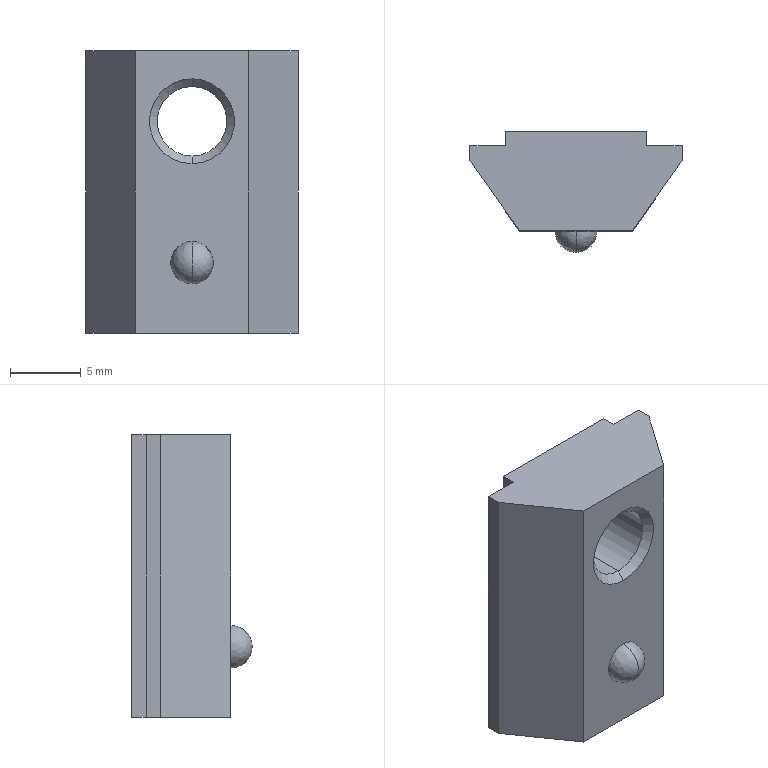Part | SolidWorks | features BaseBody 1 | 1 solid | 20 faces | box 15 x 8.5 x 20 mm | volume 1520 mm3 | plane 12 | cone 4 | spline 2 | cylinder 2 | commonest cylinder face diameters 4.917 x2
STEP:
#1=CARTESIAN_POINT('',(0.,0.,-13.5));
#2=VERTEX_POINT('',#1);
#3=CARTESIAN_POINT('',(0.,0.,-16.5));
#4=VERTEX_POINT('',#3);
#5=CARTESIAN_POINT('',(0.,0.,-15.));
#6=DIRECTION('',(0.,1.,0.));
#7=DIRECTION('',(0.,0.,1.));
#8=AXIS2_PLACEMENT_3D('',#5,#6,#7);
#9=CIRCLE('',#8,1.5);
#10=EDGE_CURVE('',#2,#4,#9,.T.);
#11=ORIENTED_EDGE('',*,*,#10,.F.);
#12=CARTESIAN_POINT('',(0.,-1.5,-15.));
#13=VERTEX_POINT('',#12);
#14=CARTESIAN_POINT('',(0.,0.,-15.));
#15=DIRECTION('',(1.,0.,0.));
#16=DIRECTION('',(0.,1.,0.));
#17=AXIS2_PLACEMENT_3D('',#14,#15,#16);
#18=CIRCLE('',#17,1.5);
#19=EDGE_CURVE('',#2,#13,#18,.T.);
#20=ORIENTED_EDGE('',*,*,#19,.T.);
#21=CARTESIAN_POINT('',(0.,0.,-15.));
#22=DIRECTION('',(-1.,0.,0.));
#23=DIRECTION('',(0.,1.,0.));
#24=AXIS2_PLACEMENT_3D('',#21,#22,#23);
#25=CIRCLE('',#24,1.5);
#26=EDGE_CURVE('',#4,#13,#25,.T.);
#27=ORIENTED_EDGE('',*,*,#26,.F.);
#28=EDGE_LOOP('',(#11,#20,#27));
#29=FACE_OUTER_BOUND('',#28,.T.);
#30=CARTESIAN_POINT('',(0.,0.,-13.5));
#31=CARTESIAN_POINT('',(3.,0.,-13.5));
#32=CARTESIAN_POINT('',(3.,0.,-16.5));
#33=CARTESIAN_POINT('',(0.,0.,-16.5));
#34=CARTESIAN_POINT('',(0.,-0.8787,-13.5));
#35=CARTESIAN_POINT('',(3.,-0.8787,-13.5));
#36=CARTESIAN_POINT('',(3.,-0.8787,-16.5));
#37=CARTESIAN_POINT('',(0.,-0.8787,-16.5));
#38=CARTESIAN_POINT('',(0.,-1.5,-14.121));
#39=CARTESIAN_POINT('',(1.757,-1.5,-14.121));
#40=CARTESIAN_POINT('',(1.757,-1.5,-15.879));
#41=CARTESIAN_POINT('',(0.,-1.5,-15.879));
#42=CARTESIAN_POINT('',(0.,-1.5,-15.));
#43=CARTESIAN_POINT('',(0.,-1.5,-15.));
#44=CARTESIAN_POINT('',(0.,-1.5,-15.));
#45=CARTESIAN_POINT('',(0.,-1.5,-15.));
#46=(BOUNDED_SURFACE()B_SPLINE_SURFACE(3,3,((#30,#31,#32,#33),(#34,#35,#36,#37),(#38,#39,#40,#41),(#42,#43,#44,#45)),.UNSPECIFIED.,.F.,.F.,.F.)B_SPLINE_SURFACE_WITH_KNOTS((4,4),(4,4),(0.,1.),(0.,1.),.UNSPECIFIED.)GEOMETRIC_REPRESENTATION_ITEM()RATIONAL_B_SPLINE_SURFACE(((1.,0.3333,0.3333,1.),(0.8047,0.2682,0.2682,0.8047),(0.8047,0.2682,0.2682,0.8047),(1.,0.3333,0.3333,1.)))REPRESENTATION_ITEM('')SURFACE());
#47=ADVANCED_FACE('',(#29),#46,.T.);
#48=CARTESIAN_POINT('',(0.,6.459,-7.458));
#49=VERTEX_POINT('',#48);
#50=CARTESIAN_POINT('',(0.,6.459,-2.542));
#51=VERTEX_POINT('',#50);
#52=CARTESIAN_POINT('',(0.,6.459,-5.));
#53=DIRECTION('',(0.,1.,0.));
#54=DIRECTION('',(0.,0.,1.));
#55=AXIS2_PLACEMENT_3D('',#52,#53,#54);
#56=CIRCLE('',#55,2.458);
#57=EDGE_CURVE('',#49,#51,#56,.T.);
#58=ORIENTED_EDGE('',*,*,#57,.F.);
#59=CARTESIAN_POINT('',(0.,7.,-8.));
#60=VERTEX_POINT('',#59);
#61=CARTESIAN_POINT('',(0.,7.,-8.));
#62=DIRECTION('',(0.,0.7071,-0.7071));
#63=VECTOR('',#62,1000.);
#64=LINE('',#61,#63);
#65=EDGE_CURVE('',#49,#60,#64,.T.);
#66=ORIENTED_EDGE('',*,*,#65,.T.);
#67=CARTESIAN_POINT('',(0.,7.,-2.));
#68=VERTEX_POINT('',#67);
#69=CARTESIAN_POINT('',(0.,7.,-5.));
#70=DIRECTION('',(0.,-1.,0.));
#71=DIRECTION('',(0.,0.,1.));
#72=AXIS2_PLACEMENT_3D('',#69,#70,#71);
#73=CIRCLE('',#72,3.);
#74=EDGE_CURVE('',#68,#60,#73,.T.);
#75=ORIENTED_EDGE('',*,*,#74,.F.);
#76=CARTESIAN_POINT('',(0.,7.,-2.));
#77=DIRECTION('',(0.,0.7071,0.7071));
#78=VECTOR('',#77,1000.);
#79=LINE('',#76,#78);
#80=EDGE_CURVE('',#51,#68,#79,.T.);
#81=ORIENTED_EDGE('',*,*,#80,.F.);
#82=EDGE_LOOP('',(#58,#66,#75,#81));
#83=FACE_OUTER_BOUND('',#82,.T.);
#84=CARTESIAN_POINT('',(0.,7.,-5.));
#85=DIRECTION('',(0.,1.,0.));
#86=DIRECTION('',(0.,0.,1.));
#87=AXIS2_PLACEMENT_3D('',#84,#85,#86);
#88=CONICAL_SURFACE('',#87,3.,0.7854);
#89=ADVANCED_FACE('',(#83),#88,.F.);
#90=CARTESIAN_POINT('',(0.,0.5415,-7.458));
#91=VERTEX_POINT('',#90);
#92=CARTESIAN_POINT('',(0.,0.5415,-2.542));
#93=VERTEX_POINT('',#92);
#94=CARTESIAN_POINT('',(0.,0.5415,-5.));
#95=DIRECTION('',(0.,1.,0.));
#96=DIRECTION('',(0.,0.,1.));
#97=AXIS2_PLACEMENT_3D('',#94,#95,#96);
#98=CIRCLE('',#97,2.458);
#99=EDGE_CURVE('',#91,#93,#98,.T.);
#100=ORIENTED_EDGE('',*,*,#99,.F.);
#101=CARTESIAN_POINT('',(0.,0.,-7.458));
#102=DIRECTION('',(0.,1.,0.));
#103=VECTOR('',#102,1000.);
#104=LINE('',#101,#103);
#105=EDGE_CURVE('',#91,#49,#104,.T.);
#106=ORIENTED_EDGE('',*,*,#105,.T.);
#107=ORIENTED_EDGE('',*,*,#57,.T.);
#108=CARTESIAN_POINT('',(0.,0.,-2.542));
#109=DIRECTION('',(0.,1.,0.));
#110=VECTOR('',#109,1000.);
#111=LINE('',#108,#110);
#112=EDGE_CURVE('',#93,#51,#111,.T.);
#113=ORIENTED_EDGE('',*,*,#112,.F.);
#114=EDGE_LOOP('',(#100,#106,#107,#113));
#115=FACE_OUTER_BOUND('',#114,.T.);
#116=CARTESIAN_POINT('',(0.,0.,-5.));
#117=DIRECTION('',(0.,1.,0.));
#118=DIRECTION('',(0.,0.,1.));
#119=AXIS2_PLACEMENT_3D('',#116,#117,#118);
#120=CYLINDRICAL_SURFACE('',#119,2.458);
#121=ADVANCED_FACE('',(#115),#120,.F.);
#122=ORIENTED_EDGE('',*,*,#99,.T.);
#123=CARTESIAN_POINT('',(0.,0.,-2.));
#124=VERTEX_POINT('',#123);
#125=CARTESIAN_POINT('',(0.,0.,-2.));
#126=DIRECTION('',(0.,-0.7071,0.7071));
#127=VECTOR('',#126,1000.);
#128=LINE('',#125,#127);
#129=EDGE_CURVE('',#93,#124,#128,.T.);
#130=ORIENTED_EDGE('',*,*,#129,.T.);
#131=CARTESIAN_POINT('',(0.,0.,-8.));
#132=VERTEX_POINT('',#131);
#133=CARTESIAN_POINT('',(0.,0.,-5.));
#134=DIRECTION('',(0.,1.,0.));
#135=DIRECTION('',(0.,0.,-1.));
#136=AXIS2_PLACEMENT_3D('',#133,#134,#135);
#137=CIRCLE('',#136,3.);
#138=EDGE_CURVE('',#132,#124,#137,.T.);
#139=ORIENTED_EDGE('',*,*,#138,.F.);
#140=CARTESIAN_POINT('',(0.,0.,-8.));
#141=DIRECTION('',(0.,-0.7071,-0.7071));
#142=VECTOR('',#141,1000.);
#143=LINE('',#140,#142);
#144=EDGE_CURVE('',#91,#132,#143,.T.);
#145=ORIENTED_EDGE('',*,*,#144,.F.);
#146=EDGE_LOOP('',(#122,#130,#139,#145));
#147=FACE_OUTER_BOUND('',#146,.T.);
#148=CARTESIAN_POINT('',(0.,0.,-5.));
#149=DIRECTION('',(0.,-1.,0.));
#150=DIRECTION('',(0.,0.,-1.));
#151=AXIS2_PLACEMENT_3D('',#148,#149,#150);
#152=CONICAL_SURFACE('',#151,3.,0.7854);
#153=ADVANCED_FACE('',(#147),#152,.F.);
#154=ORIENTED_EDGE('',*,*,#74,.T.);
#155=CARTESIAN_POINT('',(0.,7.,-5.));
#156=DIRECTION('',(0.,-1.,0.));
#157=DIRECTION('',(0.,0.,1.));
#158=AXIS2_PLACEMENT_3D('',#155,#156,#157);
#159=CIRCLE('',#158,3.);
#160=EDGE_CURVE('',#60,#68,#159,.T.);
#161=ORIENTED_EDGE('',*,*,#160,.T.);
#162=EDGE_LOOP('',(#154,#161));
#163=FACE_BOUND('',#162,.T.);
#164=CARTESIAN_POINT('',(5.,7.,-20.));
#165=VERTEX_POINT('',#164);
#166=CARTESIAN_POINT('',(-5.,7.,-20.));
#167=VERTEX_POINT('',#166);
#168=CARTESIAN_POINT('',(5.,7.,-20.));
#169=DIRECTION('',(-1.,0.,0.));
#170=VECTOR('',#169,1000.);
#171=LINE('',#168,#170);
#172=EDGE_CURVE('',#165,#167,#171,.T.);
#173=ORIENTED_EDGE('',*,*,#172,.T.);
#174=CARTESIAN_POINT('',(-5.,7.,0.));
#175=VERTEX_POINT('',#174);
#176=CARTESIAN_POINT('',(-5.,7.,-20.));
#177=DIRECTION('',(0.,0.,1.));
#178=VECTOR('',#177,1000.);
#179=LINE('',#176,#178);
#180=EDGE_CURVE('',#167,#175,#179,.T.);
#181=ORIENTED_EDGE('',*,*,#180,.T.);
#182=CARTESIAN_POINT('',(5.,7.,0.));
#183=VERTEX_POINT('',#182);
#184=CARTESIAN_POINT('',(5.,7.,0.));
#185=DIRECTION('',(1.,0.,0.));
#186=VECTOR('',#185,1000.);
#187=LINE('',#184,#186);
#188=EDGE_CURVE('',#175,#183,#187,.T.);
#189=ORIENTED_EDGE('',*,*,#188,.T.);
#190=CARTESIAN_POINT('',(5.,7.,-20.));
#191=DIRECTION('',(0.,0.,-1.));
#192=VECTOR('',#191,1000.);
#193=LINE('',#190,#192);
#194=EDGE_CURVE('',#183,#165,#193,.T.);
#195=ORIENTED_EDGE('',*,*,#194,.T.);
#196=EDGE_LOOP('',(#173,#181,#189,#195));
#197=FACE_OUTER_BOUND('',#196,.T.);
#198=CARTESIAN_POINT('',(5.,7.,-20.));
#199=DIRECTION('',(0.,1.,0.));
#200=DIRECTION('',(0.,0.,1.));
#201=AXIS2_PLACEMENT_3D('',#198,#199,#200);
#202=PLANE('',#201);
#203=ADVANCED_FACE('',(#163,#197),#202,.T.);
#204=ORIENTED_EDGE('',*,*,#65,.F.);
#205=CARTESIAN_POINT('',(0.,6.459,-5.));
#206=DIRECTION('',(0.,1.,0.));
#207=DIRECTION('',(0.,0.,1.));
#208=AXIS2_PLACEMENT_3D('',#205,#206,#207);
#209=CIRCLE('',#208,2.458);
#210=EDGE_CURVE('',#51,#49,#209,.T.);
#211=ORIENTED_EDGE('',*,*,#210,.F.);
#212=ORIENTED_EDGE('',*,*,#80,.T.);
#213=ORIENTED_EDGE('',*,*,#160,.F.);
#214=EDGE_LOOP('',(#204,#211,#212,#213));
#215=FACE_OUTER_BOUND('',#214,.T.);
#216=CARTESIAN_POINT('',(0.,7.,-5.));
#217=DIRECTION('',(0.,1.,0.));
#218=DIRECTION('',(0.,0.,1.));
#219=AXIS2_PLACEMENT_3D('',#216,#217,#218);
#220=CONICAL_SURFACE('',#219,3.,0.7854);
#221=ADVANCED_FACE('',(#215),#220,.F.);
#222=CARTESIAN_POINT('',(-5.,6.,-20.));
#223=VERTEX_POINT('',#222);
#224=CARTESIAN_POINT('',(-5.,7.,-20.));
#225=DIRECTION('',(0.,-1.,0.));
#226=VECTOR('',#225,1000.);
#227=LINE('',#224,#226);
#228=EDGE_CURVE('',#167,#223,#227,.T.);
#229=ORIENTED_EDGE('',*,*,#228,.T.);
#230=CARTESIAN_POINT('',(-5.,6.,0.));
#231=VERTEX_POINT('',#230);
#232=CARTESIAN_POINT('',(-5.,6.,-20.));
#233=DIRECTION('',(0.,0.,1.));
#234=VECTOR('',#233,1000.);
#235=LINE('',#232,#234);
#236=EDGE_CURVE('',#223,#231,#235,.T.);
#237=ORIENTED_EDGE('',*,*,#236,.T.);
#238=CARTESIAN_POINT('',(-5.,7.,0.));
#239=DIRECTION('',(0.,1.,0.));
#240=VECTOR('',#239,1000.);
#241=LINE('',#238,#240);
#242=EDGE_CURVE('',#231,#175,#241,.T.);
#243=ORIENTED_EDGE('',*,*,#242,.T.);
#244=ORIENTED_EDGE('',*,*,#180,.F.);
#245=EDGE_LOOP('',(#229,#237,#243,#244));
#246=FACE_OUTER_BOUND('',#245,.T.);
#247=CARTESIAN_POINT('',(-5.,7.,-20.));
#248=DIRECTION('',(-1.,0.,0.));
#249=DIRECTION('',(0.,0.,1.));
#250=AXIS2_PLACEMENT_3D('',#247,#248,#249);
#251=PLANE('',#250);
#252=ADVANCED_FACE('',(#246),#251,.T.);
#253=CARTESIAN_POINT('',(-7.5,6.,-20.));
#254=VERTEX_POINT('',#253);
#255=CARTESIAN_POINT('',(0.,6.,-20.));
#256=DIRECTION('',(-1.,0.,0.));
#257=VECTOR('',#256,1000.);
#258=LINE('',#255,#257);
#259=EDGE_CURVE('',#223,#254,#258,.T.);
#260=ORIENTED_EDGE('',*,*,#259,.F.);
#261=ORIENTED_EDGE('',*,*,#228,.F.);
#262=ORIENTED_EDGE('',*,*,#172,.F.);
#263=CARTESIAN_POINT('',(5.,6.,-20.));
#264=VERTEX_POINT('',#263);
#265=CARTESIAN_POINT('',(5.,0.,-20.));
#266=DIRECTION('',(0.,1.,0.));
#267=VECTOR('',#266,1000.);
#268=LINE('',#265,#267);
#269=EDGE_CURVE('',#264,#165,#268,.T.);
#270=ORIENTED_EDGE('',*,*,#269,.F.);
#271=CARTESIAN_POINT('',(7.5,6.,-20.));
#272=VERTEX_POINT('',#271);
#273=CARTESIAN_POINT('',(0.,6.,-20.));
#274=DIRECTION('',(-1.,0.,0.));
#275=VECTOR('',#274,1000.);
#276=LINE('',#273,#275);
#277=EDGE_CURVE('',#272,#264,#276,.T.);
#278=ORIENTED_EDGE('',*,*,#277,.F.);
#279=CARTESIAN_POINT('',(7.5,4.979,-20.));
#280=VERTEX_POINT('',#279);
#281=CARTESIAN_POINT('',(7.5,4.979,-20.));
#282=DIRECTION('',(0.,1.,0.));
#283=VECTOR('',#282,1000.);
#284=LINE('',#281,#283);
#285=EDGE_CURVE('',#280,#272,#284,.T.);
#286=ORIENTED_EDGE('',*,*,#285,.F.);
#287=CARTESIAN_POINT('',(4.,0.,-20.));
#288=VERTEX_POINT('',#287);
#289=CARTESIAN_POINT('',(4.,0.,-20.));
#290=DIRECTION('',(0.5751,0.8181,0.));
#291=VECTOR('',#290,1000.);
#292=LINE('',#289,#291);
#293=EDGE_CURVE('',#288,#280,#292,.T.);
#294=ORIENTED_EDGE('',*,*,#293,.F.);
#295=CARTESIAN_POINT('',(-4.,0.,-20.));
#296=VERTEX_POINT('',#295);
#297=CARTESIAN_POINT('',(0.,0.,-20.));
#298=DIRECTION('',(1.,0.,0.));
#299=VECTOR('',#298,1000.);
#300=LINE('',#297,#299);
#301=EDGE_CURVE('',#296,#288,#300,.T.);
#302=ORIENTED_EDGE('',*,*,#301,.F.);
#303=CARTESIAN_POINT('',(-7.5,5.,-20.));
#304=VERTEX_POINT('',#303);
#305=CARTESIAN_POINT('',(-7.5,5.,-20.));
#306=DIRECTION('',(0.5735,-0.8192,0.));
#307=VECTOR('',#306,1000.);
#308=LINE('',#305,#307);
#309=EDGE_CURVE('',#304,#296,#308,.T.);
#310=ORIENTED_EDGE('',*,*,#309,.F.);
#311=CARTESIAN_POINT('',(-7.5,6.,-20.));
#312=DIRECTION('',(0.,-1.,0.));
#313=VECTOR('',#312,1000.);
#314=LINE('',#311,#313);
#315=EDGE_CURVE('',#254,#304,#314,.T.);
#316=ORIENTED_EDGE('',*,*,#315,.F.);
#317=EDGE_LOOP('',(#260,#261,#262,#270,#278,#286,#294,#302,#310,#316));
#318=FACE_OUTER_BOUND('',#317,.T.);
#319=CARTESIAN_POINT('',(0.,0.,-20.));
#320=DIRECTION('',(0.,0.,1.));
#321=DIRECTION('',(1.,0.,0.));
#322=AXIS2_PLACEMENT_3D('',#319,#320,#321);
#323=PLANE('',#322);
#324=ADVANCED_FACE('',(#318),#323,.F.);
#325=ORIENTED_EDGE('',*,*,#269,.T.);
#326=ORIENTED_EDGE('',*,*,#194,.F.);
#327=CARTESIAN_POINT('',(5.,6.,0.));
#328=VERTEX_POINT('',#327);
#329=CARTESIAN_POINT('',(5.,6.,0.));
#330=DIRECTION('',(0.,-1.,0.));
#331=VECTOR('',#330,1000.);
#332=LINE('',#329,#331);
#333=EDGE_CURVE('',#183,#328,#332,.T.);
#334=ORIENTED_EDGE('',*,*,#333,.T.);
#335=CARTESIAN_POINT('',(5.,6.,-20.));
#336=DIRECTION('',(0.,0.,-1.));
#337=VECTOR('',#336,1000.);
#338=LINE('',#335,#337);
#339=EDGE_CURVE('',#328,#264,#338,.T.);
#340=ORIENTED_EDGE('',*,*,#339,.T.);
#341=EDGE_LOOP('',(#325,#326,#334,#340));
#342=FACE_OUTER_BOUND('',#341,.T.);
#343=CARTESIAN_POINT('',(5.,6.,-20.));
#344=DIRECTION('',(1.,0.,0.));
#345=DIRECTION('',(0.,0.,-1.));
#346=AXIS2_PLACEMENT_3D('',#343,#344,#345);
#347=PLANE('',#346);
#348=ADVANCED_FACE('',(#342),#347,.T.);
#349=ORIENTED_EDGE('',*,*,#242,.F.);
#350=CARTESIAN_POINT('',(-7.5,6.,0.));
#351=VERTEX_POINT('',#350);
#352=CARTESIAN_POINT('',(0.,6.,0.));
#353=DIRECTION('',(-1.,0.,0.));
#354=VECTOR('',#353,1000.);
#355=LINE('',#352,#354);
#356=EDGE_CURVE('',#231,#351,#355,.T.);
#357=ORIENTED_EDGE('',*,*,#356,.T.);
#358=CARTESIAN_POINT('',(-7.5,5.,0.));
#359=VERTEX_POINT('',#358);
#360=CARTESIAN_POINT('',(-7.5,6.,0.));
#361=DIRECTION('',(0.,1.,0.));
#362=VECTOR('',#361,1000.);
#363=LINE('',#360,#362);
#364=EDGE_CURVE('',#359,#351,#363,.T.);
#365=ORIENTED_EDGE('',*,*,#364,.F.);
#366=CARTESIAN_POINT('',(-4.,0.,0.));
#367=VERTEX_POINT('',#366);
#368=CARTESIAN_POINT('',(-7.5,5.,0.));
#369=DIRECTION('',(0.5735,-0.8192,0.));
#370=VECTOR('',#369,1000.);
#371=LINE('',#368,#370);
#372=EDGE_CURVE('',#359,#367,#371,.T.);
#373=ORIENTED_EDGE('',*,*,#372,.T.);
#374=CARTESIAN_POINT('',(4.,0.,0.));
#375=VERTEX_POINT('',#374);
#376=CARTESIAN_POINT('',(0.,0.,0.));
#377=DIRECTION('',(1.,0.,0.));
#378=VECTOR('',#377,1000.);
#379=LINE('',#376,#378);
#380=EDGE_CURVE('',#367,#375,#379,.T.);
#381=ORIENTED_EDGE('',*,*,#380,.T.);
#382=CARTESIAN_POINT('',(7.5,4.979,0.));
#383=VERTEX_POINT('',#382);
#384=CARTESIAN_POINT('',(4.,0.,0.));
#385=DIRECTION('',(0.5751,0.8181,0.));
#386=VECTOR('',#385,1000.);
#387=LINE('',#384,#386);
#388=EDGE_CURVE('',#375,#383,#387,.T.);
#389=ORIENTED_EDGE('',*,*,#388,.T.);
#390=CARTESIAN_POINT('',(7.5,6.,0.));
#391=VERTEX_POINT('',#390);
#392=CARTESIAN_POINT('',(7.5,4.979,0.));
#393=DIRECTION('',(0.,-1.,0.));
#394=VECTOR('',#393,1000.);
#395=LINE('',#392,#394);
#396=EDGE_CURVE('',#391,#383,#395,.T.);
#397=ORIENTED_EDGE('',*,*,#396,.F.);
#398=CARTESIAN_POINT('',(0.,6.,0.));
#399=DIRECTION('',(-1.,0.,0.));
#400=VECTOR('',#399,1000.);
#401=LINE('',#398,#400);
#402=EDGE_CURVE('',#391,#328,#401,.T.);
#403=ORIENTED_EDGE('',*,*,#402,.T.);
#404=ORIENTED_EDGE('',*,*,#333,.F.);
#405=ORIENTED_EDGE('',*,*,#188,.F.);
#406=EDGE_LOOP('',(#349,#357,#365,#373,#381,#389,#397,#403,#404,#405));
#407=FACE_OUTER_BOUND('',#406,.T.);
#408=CARTESIAN_POINT('',(0.,0.,0.));
#409=DIRECTION('',(0.,0.,1.));
#410=DIRECTION('',(1.,0.,0.));
#411=AXIS2_PLACEMENT_3D('',#408,#409,#410);
#412=PLANE('',#411);
#413=ADVANCED_FACE('',(#407),#412,.T.);
#414=ORIENTED_EDGE('',*,*,#105,.F.);
#415=CARTESIAN_POINT('',(0.,0.5415,-5.));
#416=DIRECTION('',(0.,1.,0.));
#417=DIRECTION('',(0.,0.,1.));
#418=AXIS2_PLACEMENT_3D('',#415,#416,#417);
#419=CIRCLE('',#418,2.458);
#420=EDGE_CURVE('',#93,#91,#419,.T.);
#421=ORIENTED_EDGE('',*,*,#420,.F.);
#422=ORIENTED_EDGE('',*,*,#112,.T.);
#423=ORIENTED_EDGE('',*,*,#210,.T.);
#424=EDGE_LOOP('',(#414,#421,#422,#423));
#425=FACE_OUTER_BOUND('',#424,.T.);
#426=CARTESIAN_POINT('',(0.,0.,-5.));
#427=DIRECTION('',(0.,1.,0.));
#428=DIRECTION('',(0.,0.,1.));
#429=AXIS2_PLACEMENT_3D('',#426,#427,#428);
#430=CYLINDRICAL_SURFACE('',#429,2.458);
#431=ADVANCED_FACE('',(#425),#430,.F.);
#432=ORIENTED_EDGE('',*,*,#259,.T.);
#433=CARTESIAN_POINT('',(-7.5,6.,-20.));
#434=DIRECTION('',(0.,0.,1.));
#435=VECTOR('',#434,1000.);
#436=LINE('',#433,#435);
#437=EDGE_CURVE('',#254,#351,#436,.T.);
#438=ORIENTED_EDGE('',*,*,#437,.T.);
#439=ORIENTED_EDGE('',*,*,#356,.F.);
#440=ORIENTED_EDGE('',*,*,#236,.F.);
#441=EDGE_LOOP('',(#432,#438,#439,#440));
#442=FACE_OUTER_BOUND('',#441,.T.);
#443=CARTESIAN_POINT('',(-5.,6.,-20.));
#444=DIRECTION('',(0.,1.,0.));
#445=DIRECTION('',(0.,0.,1.));
#446=AXIS2_PLACEMENT_3D('',#443,#444,#445);
#447=PLANE('',#446);
#448=ADVANCED_FACE('',(#442),#447,.T.);
#449=ORIENTED_EDGE('',*,*,#277,.T.);
#450=ORIENTED_EDGE('',*,*,#339,.F.);
#451=ORIENTED_EDGE('',*,*,#402,.F.);
#452=CARTESIAN_POINT('',(7.5,6.,-20.));
#453=DIRECTION('',(0.,0.,-1.));
#454=VECTOR('',#453,1000.);
#455=LINE('',#452,#454);
#456=EDGE_CURVE('',#391,#272,#455,.T.);
#457=ORIENTED_EDGE('',*,*,#456,.T.);
#458=EDGE_LOOP('',(#449,#450,#451,#457));
#459=FACE_OUTER_BOUND('',#458,.T.);
#460=CARTESIAN_POINT('',(7.5,6.,-20.));
#461=DIRECTION('',(0.,1.,0.));
#462=DIRECTION('',(0.,0.,1.));
#463=AXIS2_PLACEMENT_3D('',#460,#461,#462);
#464=PLANE('',#463);
#465=ADVANCED_FACE('',(#459),#464,.T.);
#466=ORIENTED_EDGE('',*,*,#293,.T.);
#467=CARTESIAN_POINT('',(7.5,4.979,-20.));
#468=DIRECTION('',(0.,0.,1.));
#469=VECTOR('',#468,1000.);
#470=LINE('',#467,#469);
#471=EDGE_CURVE('',#280,#383,#470,.T.);
#472=ORIENTED_EDGE('',*,*,#471,.T.);
#473=ORIENTED_EDGE('',*,*,#388,.F.);
#474=CARTESIAN_POINT('',(4.,0.,-20.));
#475=DIRECTION('',(0.,0.,-1.));
#476=VECTOR('',#475,1000.);
#477=LINE('',#474,#476);
#478=EDGE_CURVE('',#375,#288,#477,.T.);
#479=ORIENTED_EDGE('',*,*,#478,.T.);
#480=EDGE_LOOP('',(#466,#472,#473,#479));
#481=FACE_OUTER_BOUND('',#480,.T.);
#482=CARTESIAN_POINT('',(4.,0.,-20.));
#483=DIRECTION('',(0.8181,-0.5751,0.));
#484=DIRECTION('',(0.5751,0.8181,0.));
#485=AXIS2_PLACEMENT_3D('',#482,#483,#484);
#486=PLANE('',#485);
#487=ADVANCED_FACE('',(#481),#486,.T.);
#488=ORIENTED_EDGE('',*,*,#138,.T.);
#489=CARTESIAN_POINT('',(0.,0.,-5.));
#490=DIRECTION('',(0.,1.,0.));
#491=DIRECTION('',(0.,0.,-1.));
#492=AXIS2_PLACEMENT_3D('',#489,#490,#491);
#493=CIRCLE('',#492,3.);
#494=EDGE_CURVE('',#124,#132,#493,.T.);
#495=ORIENTED_EDGE('',*,*,#494,.T.);
#496=EDGE_LOOP('',(#488,#495));
#497=FACE_BOUND('',#496,.T.);
#498=ORIENTED_EDGE('',*,*,#301,.T.);
#499=ORIENTED_EDGE('',*,*,#478,.F.);
#500=ORIENTED_EDGE('',*,*,#380,.F.);
#501=CARTESIAN_POINT('',(-4.,0.,-20.));
#502=DIRECTION('',(0.,0.,-1.));
#503=VECTOR('',#502,1000.);
#504=LINE('',#501,#503);
#505=EDGE_CURVE('',#367,#296,#504,.T.);
#506=ORIENTED_EDGE('',*,*,#505,.T.);
#507=EDGE_LOOP('',(#498,#499,#500,#506));
#508=FACE_OUTER_BOUND('',#507,.T.);
#509=CARTESIAN_POINT('',(0.,0.,-15.));
#510=DIRECTION('',(0.,1.,0.));
#511=DIRECTION('',(0.,0.,1.));
#512=AXIS2_PLACEMENT_3D('',#509,#510,#511);
#513=CIRCLE('',#512,1.5);
#514=EDGE_CURVE('',#4,#2,#513,.T.);
#515=ORIENTED_EDGE('',*,*,#514,.T.);
#516=ORIENTED_EDGE('',*,*,#10,.T.);
#517=EDGE_LOOP('',(#515,#516));
#518=FACE_BOUND('',#517,.T.);
#519=CARTESIAN_POINT('',(-4.,0.,-20.));
#520=DIRECTION('',(0.,-1.,0.));
#521=DIRECTION('',(0.,0.,-1.));
#522=AXIS2_PLACEMENT_3D('',#519,#520,#521);
#523=PLANE('',#522);
#524=ADVANCED_FACE('',(#497,#508,#518),#523,.T.);
#525=ORIENTED_EDGE('',*,*,#309,.T.);
#526=ORIENTED_EDGE('',*,*,#505,.F.);
#527=ORIENTED_EDGE('',*,*,#372,.F.);
#528=CARTESIAN_POINT('',(-7.5,5.,-20.));
#529=DIRECTION('',(0.,0.,-1.));
#530=VECTOR('',#529,1000.);
#531=LINE('',#528,#530);
#532=EDGE_CURVE('',#359,#304,#531,.T.);
#533=ORIENTED_EDGE('',*,*,#532,.T.);
#534=EDGE_LOOP('',(#525,#526,#527,#533));
#535=FACE_OUTER_BOUND('',#534,.T.);
#536=CARTESIAN_POINT('',(-7.5,5.,-20.));
#537=DIRECTION('',(-0.8192,-0.5735,0.));
#538=DIRECTION('',(0.5735,-0.8192,0.));
#539=AXIS2_PLACEMENT_3D('',#536,#537,#538);
#540=PLANE('',#539);
#541=ADVANCED_FACE('',(#535),#540,.T.);
#542=ORIENTED_EDGE('',*,*,#129,.F.);
#543=ORIENTED_EDGE('',*,*,#420,.T.);
#544=ORIENTED_EDGE('',*,*,#144,.T.);
#545=ORIENTED_EDGE('',*,*,#494,.F.);
#546=EDGE_LOOP('',(#542,#543,#544,#545));
#547=FACE_OUTER_BOUND('',#546,.T.);
#548=CARTESIAN_POINT('',(0.,0.,-5.));
#549=DIRECTION('',(0.,-1.,0.));
#550=DIRECTION('',(0.,0.,-1.));
#551=AXIS2_PLACEMENT_3D('',#548,#549,#550);
#552=CONICAL_SURFACE('',#551,3.,0.7854);
#553=ADVANCED_FACE('',(#547),#552,.F.);
#554=ORIENTED_EDGE('',*,*,#315,.T.);
#555=ORIENTED_EDGE('',*,*,#532,.F.);
#556=ORIENTED_EDGE('',*,*,#364,.T.);
#557=ORIENTED_EDGE('',*,*,#437,.F.);
#558=EDGE_LOOP('',(#554,#555,#556,#557));
#559=FACE_OUTER_BOUND('',#558,.T.);
#560=CARTESIAN_POINT('',(-7.5,6.,-20.));
#561=DIRECTION('',(-1.,0.,0.));
#562=DIRECTION('',(0.,0.,1.));
#563=AXIS2_PLACEMENT_3D('',#560,#561,#562);
#564=PLANE('',#563);
#565=ADVANCED_FACE('',(#559),#564,.T.);
#566=ORIENTED_EDGE('',*,*,#285,.T.);
#567=ORIENTED_EDGE('',*,*,#456,.F.);
#568=ORIENTED_EDGE('',*,*,#396,.T.);
#569=ORIENTED_EDGE('',*,*,#471,.F.);
#570=EDGE_LOOP('',(#566,#567,#568,#569));
#571=FACE_OUTER_BOUND('',#570,.T.);
#572=CARTESIAN_POINT('',(7.5,4.979,-20.));
#573=DIRECTION('',(1.,0.,0.));
#574=DIRECTION('',(0.,0.,-1.));
#575=AXIS2_PLACEMENT_3D('',#572,#573,#574);
#576=PLANE('',#575);
#577=ADVANCED_FACE('',(#571),#576,.T.);
#578=ORIENTED_EDGE('',*,*,#19,.F.);
#579=ORIENTED_EDGE('',*,*,#514,.F.);
#580=ORIENTED_EDGE('',*,*,#26,.T.);
#581=EDGE_LOOP('',(#578,#579,#580));
#582=FACE_OUTER_BOUND('',#581,.T.);
#583=CARTESIAN_POINT('',(0.,0.,-16.5));
#584=CARTESIAN_POINT('',(-3.,0.,-16.5));
#585=CARTESIAN_POINT('',(-3.,0.,-13.5));
#586=CARTESIAN_POINT('',(0.,0.,-13.5));
#587=CARTESIAN_POINT('',(0.,-0.8787,-16.5));
#588=CARTESIAN_POINT('',(-3.,-0.8787,-16.5));
#589=CARTESIAN_POINT('',(-3.,-0.8787,-13.5));
#590=CARTESIAN_POINT('',(0.,-0.8787,-13.5));
#591=CARTESIAN_POINT('',(0.,-1.5,-15.879));
#592=CARTESIAN_POINT('',(-1.757,-1.5,-15.879));
#593=CARTESIAN_POINT('',(-1.757,-1.5,-14.121));
#594=CARTESIAN_POINT('',(0.,-1.5,-14.121));
#595=CARTESIAN_POINT('',(0.,-1.5,-15.));
#596=CARTESIAN_POINT('',(0.,-1.5,-15.));
#597=CARTESIAN_POINT('',(0.,-1.5,-15.));
#598=CARTESIAN_POINT('',(0.,-1.5,-15.));
#599=(BOUNDED_SURFACE()B_SPLINE_SURFACE(3,3,((#583,#584,#585,#586),(#587,#588,#589,#590),(#591,#592,#593,#594),(#595,#596,#597,#598)),.UNSPECIFIED.,.F.,.F.,.F.)B_SPLINE_SURFACE_WITH_KNOTS((4,4),(4,4),(0.,1.),(0.,1.),.UNSPECIFIED.)GEOMETRIC_REPRESENTATION_ITEM()RATIONAL_B_SPLINE_SURFACE(((1.,0.3333,0.3333,1.),(0.8047,0.2682,0.2682,0.8047),(0.8047,0.2682,0.2682,0.8047),(1.,0.3333,0.3333,1.)))REPRESENTATION_ITEM('')SURFACE());
#600=ADVANCED_FACE('',(#582),#599,.T.);
#601=CLOSED_SHELL('',(#47,#89,#121,#153,#203,#221,#252,#324,#348,#413,#431,#448,#465,#487,#524,#541,#553,#565,#577,#600));
#602=MANIFOLD_SOLID_BREP('',#601);
#603=CARTESIAN_POINT('',(0.,0.,0.));
#604=DIRECTION('',(0.,0.,1.));
#605=DIRECTION('',(1.,0.,0.));
#606=AXIS2_PLACEMENT_3D('',#603,#604,#605);
#607=(LENGTH_UNIT()NAMED_UNIT(*)SI_UNIT(.MILLI.,.METRE.));
#608=UNCERTAINTY_MEASURE_WITH_UNIT(LENGTH_MEASURE(0.00001),#607,'','');
#609=(NAMED_UNIT(*)PLANE_ANGLE_UNIT()SI_UNIT($,.RADIAN.));
#610=(NAMED_UNIT(*)SI_UNIT($,.STERADIAN.)SOLID_ANGLE_UNIT());
#611=(GEOMETRIC_REPRESENTATION_CONTEXT(3)GLOBAL_UNCERTAINTY_ASSIGNED_CONTEXT((#608))GLOBAL_UNIT_ASSIGNED_CONTEXT((#607,#609,#610))REPRESENTATION_CONTEXT('',''));
#612=ADVANCED_BREP_SHAPE_REPRESENTATION('',(#602,#606),#611);